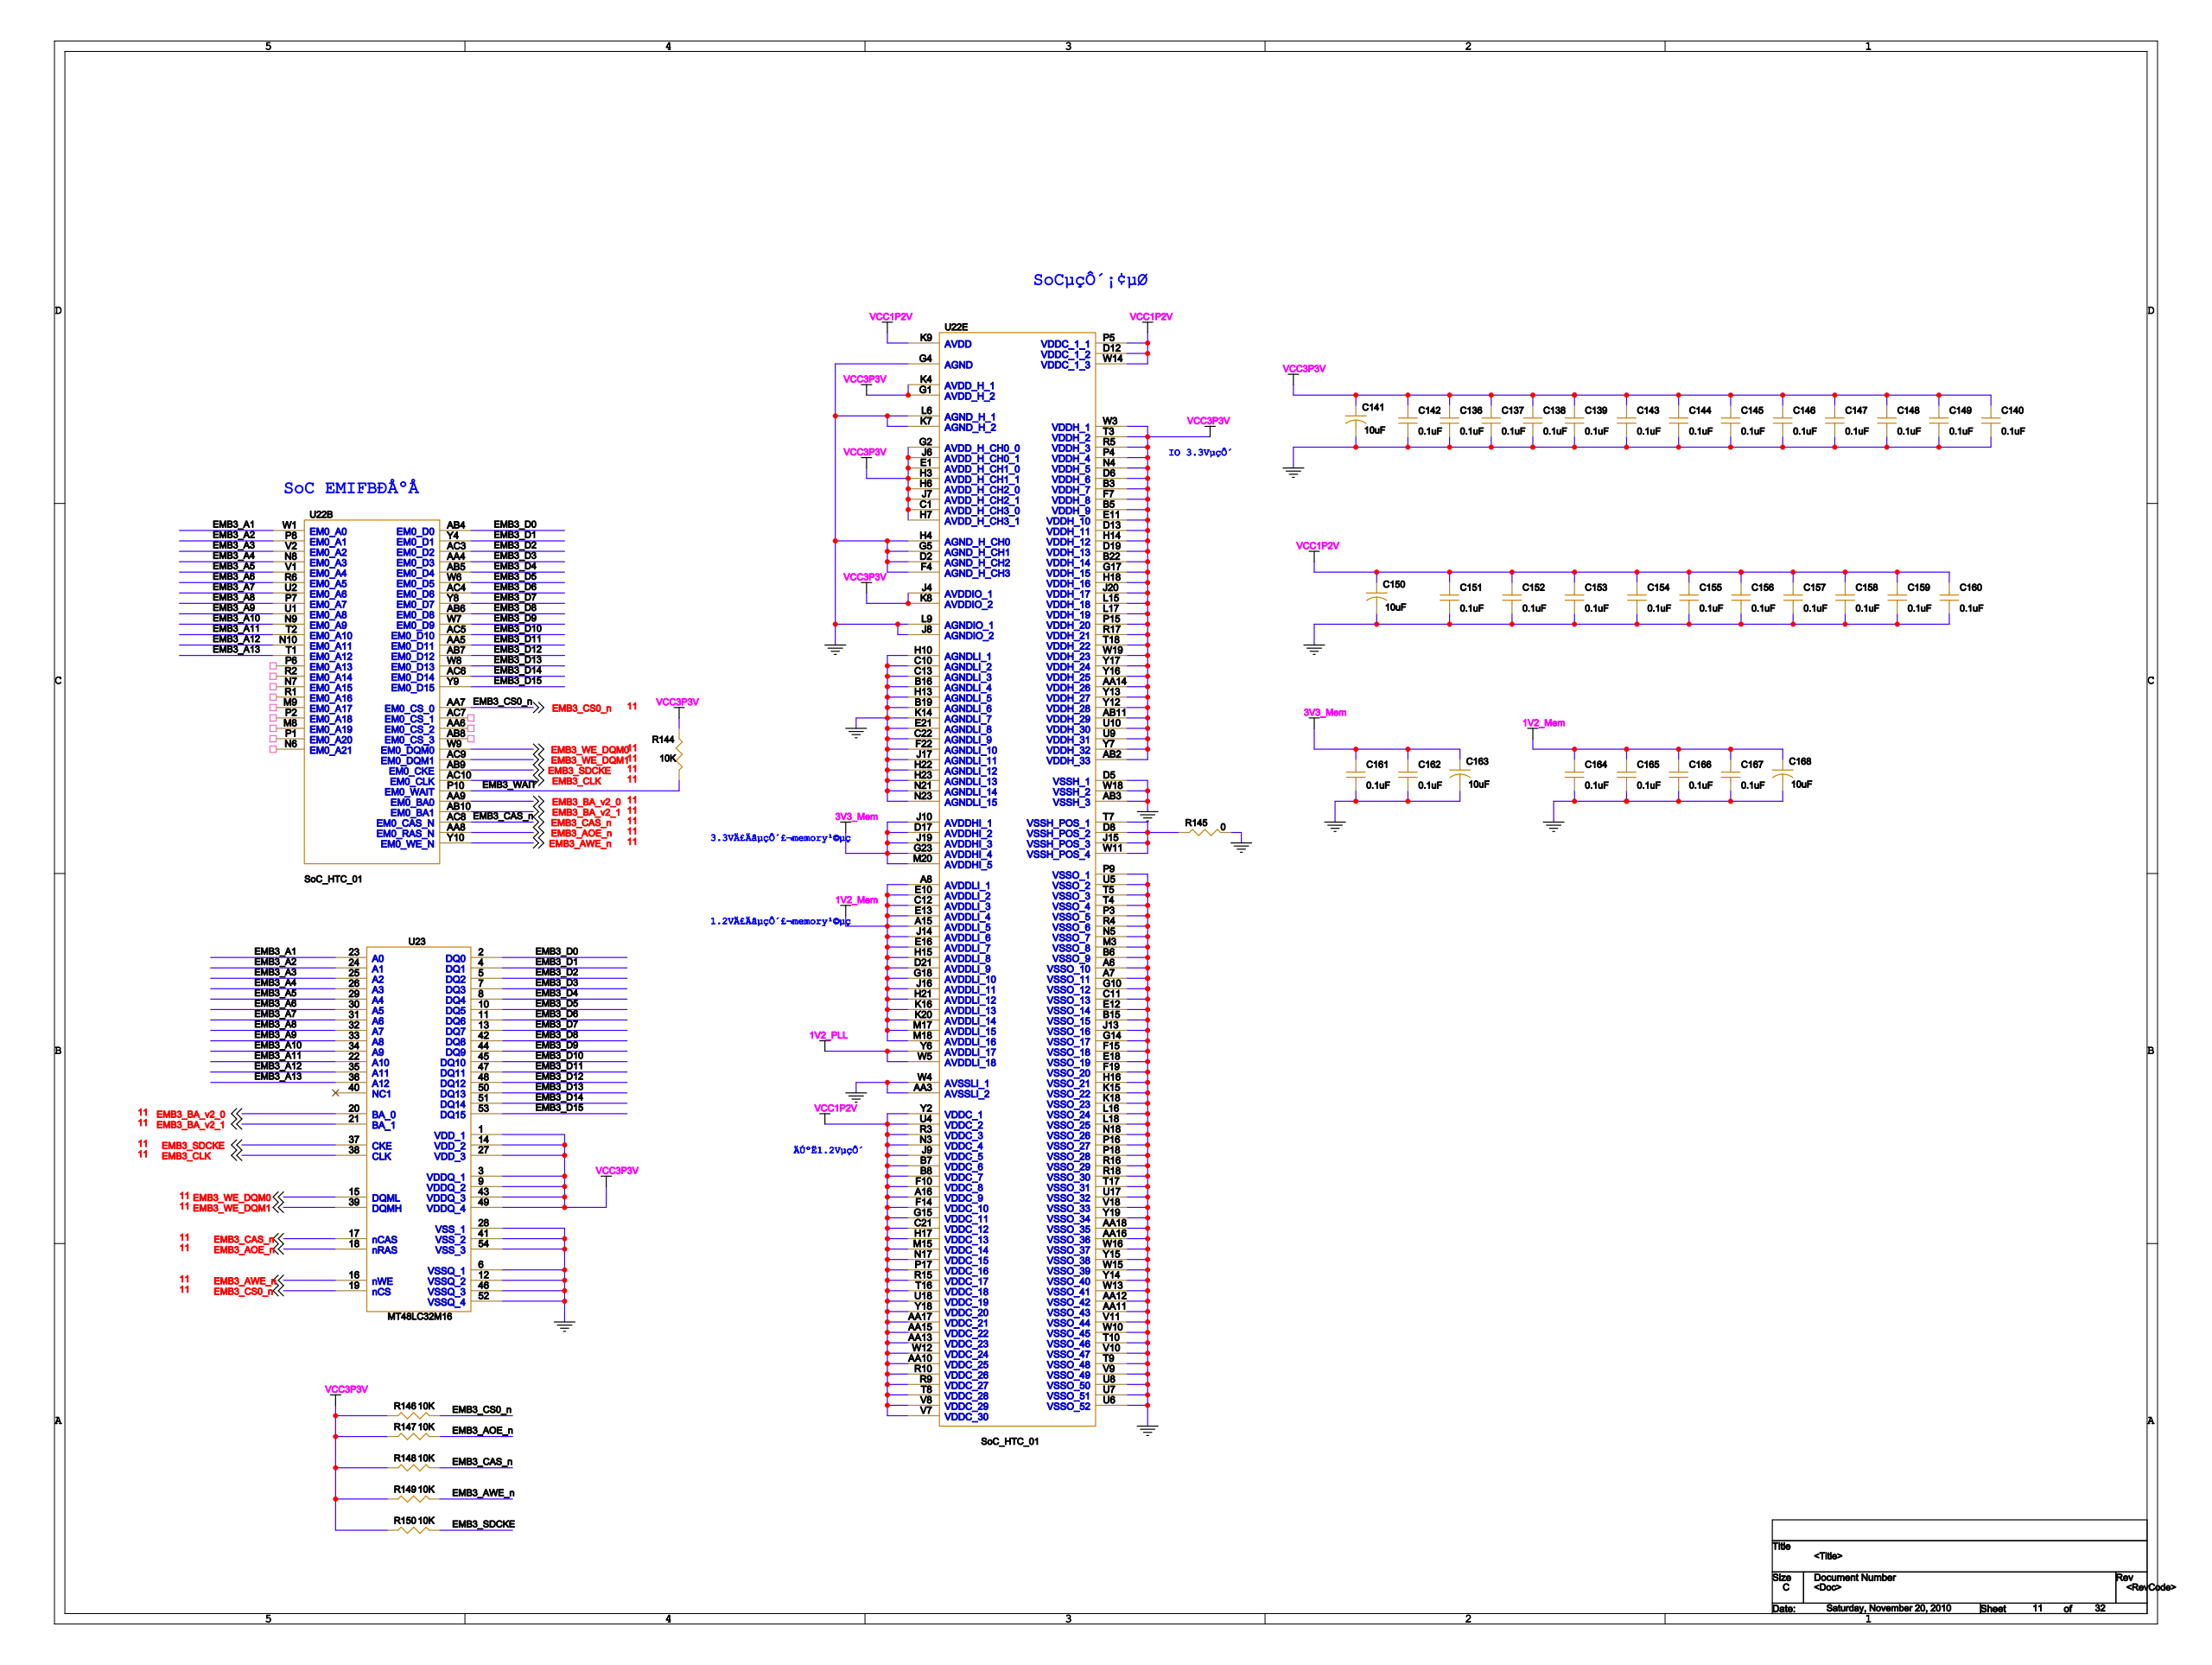Circuit board | Cadence Allegro | 1001 parts | 1318 nets | one sheet of the schematic
Parts on this sheet (reference | value | footprint):
C136 | 0.1uF | C0402
C137 | 0.1uF | C0402
C138 | 0.1uF | C0402
C139 | 0.1uF | C0402
C140 | 0.1uF | C0402
C141 | 10uF | C3216
C142 | 0.1uF | C0402
C143 | 0.1uF | C0402
C144 | 0.1uF | C0402
C145 | 0.1uF | C0402
C146 | 0.1uF | C0402
C147 | 0.1uF | C0402
C148 | 0.1uF | C0402
C149 | 0.1uF | C0402
C150 | 10uF | C3216
C151 | 0.1uF | C0402
C152 | 0.1uF | C0402
C153 | 0.1uF | C0402
C154 | 0.1uF | C0402
C155 | 0.1uF | C0402
C156 | 0.1uF | C0402
C157 | 0.1uF | C0402
C158 | 0.1uF | C0402
C159 | 0.1uF | C0402
C160 | 0.1uF | C0402
C161 | 0.1uF | C0402
C162 | 0.1uF | C0402
C163 | 10uF | C3216
C164 | 0.1uF | C0402
C165 | 0.1uF | C0402
C166 | 0.1uF | C0402
C167 | 0.1uF | C0402
C168 | 10uF | C3216
R144 | 10K | 0603
R145 | 0 | 0603
R146 | 10K | 0603
R147 | 10K | 0603
R148 | 10K | 0603
R149 | 10K | 0603
R150 | 10K | 0603
U1 | SoC_HTC_01 | L529_XIN
U2 | MT48LC32M16 | TSOP54
U4 | MAX3243 | TSSOP-28
U6 | MT48LC16M16 | TSOP54
U7 | MT48LC16M16 | TSOP54
U8 | DP83848C | DP83848C_48LQFP
U10 | SoC_HTC_01 | L529_XIN
U17 | MT48LC32M16 | TSOP54
U22 | SoC_HTC_01 | L529_XIN
U23 | MT48LC32M16 | TSOP54
Nets of these parts (net: part-pin ...):
GND: C136-2 C137-2 C138-2 C139-2 C140-2 C141-2 C142-2 C143-2 C144-2 C145-2 C146-2 C147-2 C148-2 C149-2 C150-2 C151-2 C152-2 C153-2 C154-2 C155-2 C156-2 C157-2 C158-2 C159-2 C160-2 C161-2 C162-2 C163-2 C164-2 C165-2 C166-2 C167-2 C168-2 R145-2 U1-A6 U1-A7 U1-AA3 U1-AA11 U1-AA12 U1-AA16 U1-AA18 U1-AB3 U1-B6 U1-B15 U1-B16 U1-B19 U1-C10 U1-C11 U1-C13 U1-C22 U1-D2 U1-D5 U1-E12 U1-E18 U1-E21 U1-F4 U1-F15 U1-F19 U1-F22 U1-G4 U1-G5 U1-G10 U1-G14 U1-H4 U1-H10 U1-H13 U1-H16 U1-H22 U1-H23 U1-J8 U1-J13 U1-J17 U1-K7 U1-K14 U1-K15 U1-K18 U1-L6 U1-L9 U1-L16 U1-L18 U1-M3 U1-N5 U1-N18 U1-N21 U1-N23 U1-P3 U1-P9 U1-P16 U1-P18 U1-R4 U1-R16 U1-R18 U1-T4 U1-T5 U1-T9 U1-T10 U1-T17 U1-U5 U1-U6 U1-U7 U1-U8 U1-U17 U1-V9 U1-V10 U1-V11 U1-V18 U1-W4 U1-W10 U1-W13 U1-W15 U1-W16 U1-W18 U1-Y14 U1-Y15 U1-Y19 U2-6 U2-12 U2-28 U2-41 U2-46 U2-52 U2-54 U4-23 U4-25 U6-6 U6-12 U6-28 U6-41 U6-46 U6-52 U6-54 U7-6 U7-12 U7-28 U7-41 U7-46 U7-52 U7-54 U8-15 U8-19 U8-35 U8-36 U8-47 U10-A6 U10-A7 U10-AA3 U10-AA11 U10-AA12 U10-AA16 U10-AA18 U10-AB3 U10-B6 U10-B15 U10-B16 U10-B19 U10-C10 U10-C11 U10-C13 U10-C22 U10-D2 U10-D5 U10-E12 U10-E18 U10-E21 U10-F4 U10-F15 U10-F19 U10-F22 U10-G4 U10-G5 U10-G10 U10-G14 U10-H4 U10-H10 U10-H13 U10-H16 U10-H22 U10-H23 U10-J8 U10-J13 U10-J17 U10-K7 U10-K14 U10-K15 U10-K18 U10-L6 U10-L9 U10-L16 U10-L18 U10-M3 U10-N5 U10-N18 U10-N21 U10-N23 U10-P3 U10-P9 U10-P16 U10-P18 U10-R4 U10-R16 U10-R18 U10-T4 U10-T5 U10-T9 U10-T10 U10-T17 U10-U5 U10-U6 U10-U7 U10-U8 U10-U17 U10-V9 U10-V10 U10-V11 U10-V18 U10-W4 U10-W10 U10-W13 U10-W15 U10-W16 U10-W18 U10-Y14 U10-Y15 U10-Y19 U17-6 U17-12 U17-28 U17-41 U17-46 U17-52 U17-54 U22-A6 U22-A7 U22-AA3 U22-AA11 U22-AA12 U22-AA16 U22-AA18 U22-AB3 U22-B6 U22-B15 U22-B16 U22-B19 U22-C10 U22-C11 U22-C13 U22-C22 U22-D2 U22-D5 U22-E12 U22-E18 U22-E21 U22-F4 U22-F15 U22-F19 U22-F22 U22-G4 U22-G5 U22-G10 U22-G14 U22-H4 U22-H10 U22-H13 U22-H16 U22-H22 U22-H23 U22-J8 U22-J13 U22-J17 U22-K7 U22-K14 U22-K15 U22-K18 U22-L6 U22-L9 U22-L16 U22-L18 U22-M3 U22-N5 U22-N18 U22-N21 U22-N23 U22-P3 U22-P9 U22-P16 U22-P18 U22-R4 U22-R16 U22-R18 U22-T4 U22-T5 U22-T9 U22-T10 U22-T17 U22-U5 U22-U6 U22-U7 U22-U8 U22-U17 U22-V9 U22-V10 U22-V11 U22-V18 U22-W4 U22-W10 U22-W13 U22-W15 U22-W16 U22-W18 U22-Y14 U22-Y15 U22-Y19 U23-6 U23-12 U23-28 U23-41 U23-46 U23-52 U23-54
VCC3P3V: C136-1 C137-1 C138-1 C139-1 C140-1 C141-1 C142-1 C143-1 C144-1 C145-1 C146-1 C147-1 C148-1 C149-1 R144-2 R146-1 R147-1 R148-1 R149-1 R150-1 U1-AA14 U1-AB2 U1-AB11 U1-B3 U1-B5 U1-B22 U1-C1 U1-D6 U1-D13 U1-D19 U1-E1 U1-E11 U1-F7 U1-G1 U1-G2 U1-G17 U1-H3 U1-H6 U1-H7 U1-H14 U1-H18 U1-J4 U1-J6 U1-J7 U1-J20 U1-K4 U1-K8 U1-L15 U1-L17 U1-N4 U1-P4 U1-P15 U1-R5 U1-R17 U1-T3 U1-T18 U1-U9 U1-U10 U1-W3 U1-W19 U1-Y7 U1-Y12 U1-Y13 U1-Y16 U1-Y17 U2-1 U2-3 U2-9 U2-14 U2-27 U2-43 U2-49 U4-22 U4-26 U6-1 U6-3 U6-9 U6-14 U6-27 U6-43 U6-49 U7-1 U7-3 U7-9 U7-14 U7-27 U7-43 U7-49 U8-22 U8-32 U8-48 U10-AA14 U10-AB2 U10-AB11 U10-B3 U10-B5 U10-B22 U10-C1 U10-D6 U10-D13 U10-D19 U10-E1 U10-E11 U10-F7 U10-G1 U10-G2 U10-G17 U10-H3 U10-H6 U10-H7 U10-H14 U10-H18 U10-J4 U10-J6 U10-J7 U10-J20 U10-K4 U10-K8 U10-L15 U10-L17 U10-N4 U10-P4 U10-P15 U10-R5 U10-R17 U10-T3 U10-T18 U10-U9 U10-U10 U10-W3 U10-W19 U10-Y7 U10-Y12 U10-Y13 U10-Y16 U10-Y17 U17-1 U17-3 U17-9 U17-14 U17-27 U17-43 U17-49 U22-AA14 U22-AB2 U22-AB11 U22-B3 U22-B5 U22-B22 U22-C1 U22-D6 U22-D13 U22-D19 U22-E1 U22-E11 U22-F7 U22-G1 U22-G2 U22-G17 U22-H3 U22-H6 U22-H7 U22-H14 U22-H18 U22-J4 U22-J6 U22-J7 U22-J20 U22-K4 U22-K8 U22-L15 U22-L17 U22-N4 U22-P4 U22-P15 U22-R5 U22-R17 U22-T3 U22-T18 U22-U9 U22-U10 U22-W3 U22-W19 U22-Y7 U22-Y12 U22-Y13 U22-Y16 U22-Y17 U23-1 U23-3 U23-9 U23-14 U23-27 U23-43 U23-49
VCC1P2V: C150-1 C151-1 C152-1 C153-1 C154-1 C155-1 C156-1 C157-1 C158-1 C159-1 C160-1 U1-A16 U1-AA10 U1-AA13 U1-AA15 U1-AA17 U1-B7 U1-B8 U1-C21 U1-D12 U1-F10 U1-F14 U1-G15 U1-H17 U1-J9 U1-K9 U1-M15 U1-N3 U1-N17 U1-P5 U1-P17 U1-R3 U1-R9 U1-R10 U1-R15 U1-T8 U1-T16 U1-U4 U1-U18 U1-V7 U1-V8 U1-W12 U1-W14 U1-Y2 U1-Y18 U10-A16 U10-AA10 U10-AA13 U10-AA15 U10-AA17 U10-B7 U10-B8 U10-C21 U10-D12 U10-F10 U10-F14 U10-G15 U10-H17 U10-J9 U10-K9 U10-M15 U10-N3 U10-N17 U10-P5 U10-P17 U10-R3 U10-R9 U10-R10 U10-R15 U10-T8 U10-T16 U10-U4 U10-U18 U10-V7 U10-V8 U10-W12 U10-W14 U10-Y2 U10-Y18 U22-A16 U22-AA10 U22-AA13 U22-AA15 U22-AA17 U22-B7 U22-B8 U22-C21 U22-D12 U22-F10 U22-F14 U22-G15 U22-H17 U22-J9 U22-K9 U22-M15 U22-N3 U22-N17 U22-P5 U22-P17 U22-R3 U22-R9 U22-R10 U22-R15 U22-T8 U22-T16 U22-U4 U22-U18 U22-V7 U22-V8 U22-W12 U22-W14 U22-Y2 U22-Y18
3V3_MEM: C161-1 C162-1 C163-1 U1-D17 U1-G23 U1-J10 U1-J19 U1-M20 U10-D17 U10-G23 U10-J10 U10-J19 U10-M20 U22-D17 U22-G23 U22-J10 U22-J19 U22-M20
1V2_MEM: C164-1 C165-1 C166-1 C167-1 C168-1 U1-A8 U1-A15 U1-C12 U1-D21 U1-E10 U1-E13 U1-E16 U1-G18 U1-H15 U1-H21 U1-J14 U1-J16 U1-K16 U1-K20 U1-M17 U1-M18 U10-A8 U10-A15 U10-C12 U10-D21 U10-E10 U10-E13 U10-E16 U10-G18 U10-H15 U10-H21 U10-J14 U10-J16 U10-K16 U10-K20 U10-M17 U10-M18 U22-A8 U22-A15 U22-C12 U22-D21 U22-E10 U22-E13 U22-E16 U22-G18 U22-H15 U22-H21 U22-J14 U22-J16 U22-K16 U22-K20 U22-M17 U22-M18
1V2_PLL: U1-W5 U1-Y6 U10-W5 U10-Y6 U22-W5 U22-Y6
EMB3_A1: U22-W1 U23-23
EMB3_A2: U22-P8 U23-24
EMB3_A11: U22-T2 U23-22
EMB3_A12: U22-N10 U23-35
EMB3_A13: U22-T1 U23-36
EMB3_A3: U22-V2 U23-25
EMB3_A4: U22-N8 U23-26
EMB3_A5: U22-V1 U23-29
EMB3_A6: U22-R6 U23-30
EMB3_A7: U22-U2 U23-31
EMB3_A8: U22-P7 U23-32
EMB3_A9: U22-U1 U23-33
EMB3_A10: U22-N9 U23-34
EMB3_CAS_N: R148-2 U22-AC8 U23-17
EMB3_SDCKE: R150-2 U22-AB9 U23-37
EMB3_CLK: U22-AC10 U23-38
EMB3_CS0_N: R146-2 U22-AA7 U23-19
EMB3_D0: U22-AB4 U23-2
EMB3_D1: U22-Y4 U23-4
EMB3_D10: U22-AC5 U23-45
EMB3_D11: U22-AA5 U23-47
EMB3_D12: U22-AB7 U23-48
EMB3_D13: U22-W8 U23-50
EMB3_D14: U22-AC6 U23-51
EMB3_D15: U22-Y9 U23-53
EMB3_D2: U22-AC3 U23-5
EMB3_D3: U22-AA4 U23-7
EMB3_D4: U22-AB5 U23-8
EMB3_D5: U22-W6 U23-10
EMB3_D6: U22-AC4 U23-11
EMB3_D7: U22-Y8 U23-13
EMB3_D8: U22-AB6 U23-42
EMB3_D9: U22-W7 U23-44
EMB3_WE_DQM0: U22-W9 U23-15
EMB3_WE_DQM1: U22-AC9 U23-39
EMB3_AOE_N: R147-2 U22-AA8 U23-18
EMB3_WAIT: R144-1 U22-P10
EMB3_AWE_N: R149-2 U22-Y10 U23-16
N17403902: R145-1 U22-D8 U22-J15 U22-T7 U22-W11